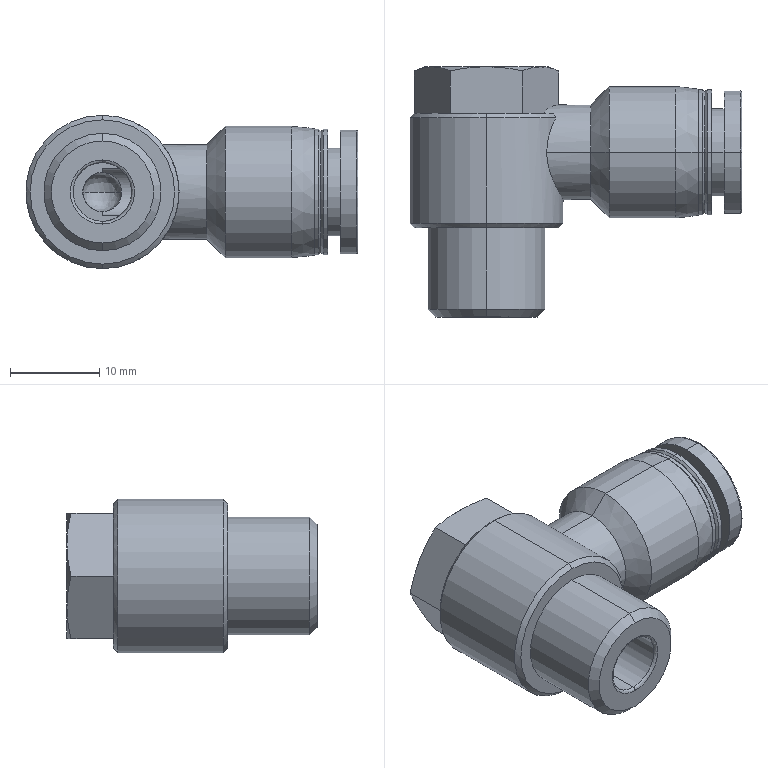Part | STEP file | External hex shaft joint APH8-02 | 1 solid | 77 faces | box 37.183 x 28 x 17.166 mm | volume 6274 mm3 | cylinder 25 | plane 23 | cone 21 | spline 8 | commonest cylinder face diameters 14.1 x4 4.386 x3 5.333 x2 6.579 x2 8 x2 9.8 x2